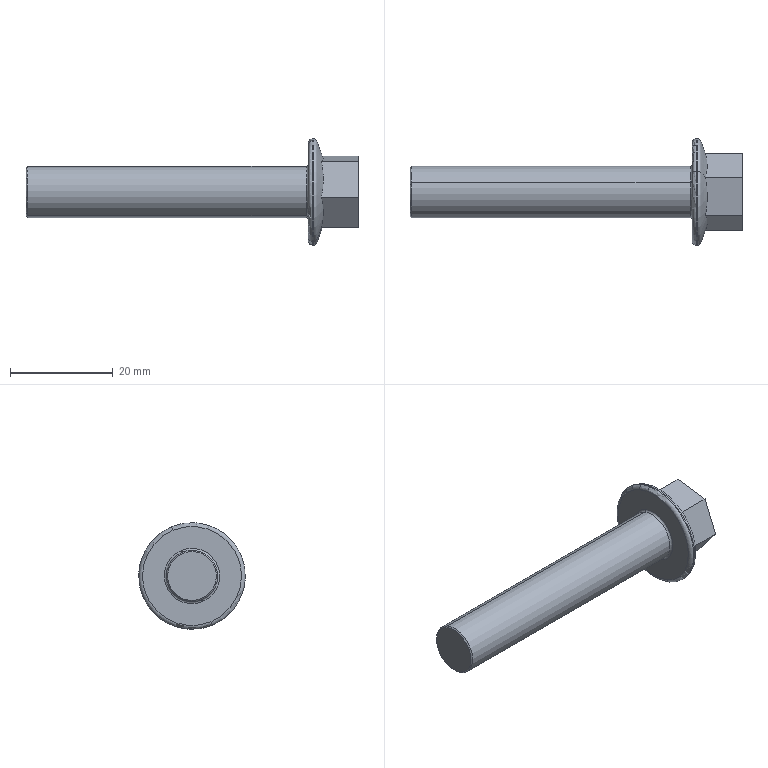Part | SolidWorks | features BaseBody 1 | 1 solid | 30 faces | box 64.7 x 20.8 x 20.8 mm | volume 6136 mm3 | cone 11 | plane 9 | torus 6 | cylinder 4 | commonest cylinder face diameters 10 x2 20.8 x2
STEP:
#1=CARTESIAN_POINT('',(181.975,42.982,433.757));
#2=VERTEX_POINT('',#1);
#3=CARTESIAN_POINT('',(181.975,35.018,414.543));
#4=VERTEX_POINT('',#3);
#5=CARTESIAN_POINT('',(181.975,39.,424.15));
#6=DIRECTION('',(-1.,0.,0.));
#7=DIRECTION('',(0.,-0.3829,-0.9238));
#8=AXIS2_PLACEMENT_3D('',#5,#6,#7);
#9=CIRCLE('',#8,10.4);
#10=EDGE_CURVE('',#2,#4,#9,.T.);
#11=ORIENTED_EDGE('',*,*,#10,.T.);
#12=CARTESIAN_POINT('',(181.75,35.018,414.543));
#13=VERTEX_POINT('',#12);
#14=CARTESIAN_POINT('',(182.5,35.018,414.543));
#15=DIRECTION('',(-1.,0.,0.));
#16=VECTOR('',#15,1000.);
#17=LINE('',#14,#16);
#18=EDGE_CURVE('',#4,#13,#17,.T.);
#19=ORIENTED_EDGE('',*,*,#18,.T.);
#20=CARTESIAN_POINT('',(181.75,42.982,433.757));
#21=VERTEX_POINT('',#20);
#22=CARTESIAN_POINT('',(181.75,39.,424.15));
#23=DIRECTION('',(1.,0.,0.));
#24=DIRECTION('',(0.,0.3829,0.9238));
#25=AXIS2_PLACEMENT_3D('',#22,#23,#24);
#26=CIRCLE('',#25,10.4);
#27=EDGE_CURVE('',#13,#21,#26,.T.);
#28=ORIENTED_EDGE('',*,*,#27,.T.);
#29=CARTESIAN_POINT('',(182.5,42.982,433.757));
#30=DIRECTION('',(-1.,0.,0.));
#31=VECTOR('',#30,1000.);
#32=LINE('',#29,#31);
#33=EDGE_CURVE('',#2,#21,#32,.T.);
#34=ORIENTED_EDGE('',*,*,#33,.F.);
#35=EDGE_LOOP('',(#11,#19,#28,#34));
#36=FACE_OUTER_BOUND('',#35,.T.);
#37=CARTESIAN_POINT('',(182.5,39.,424.15));
#38=DIRECTION('',(-1.,0.,0.));
#39=DIRECTION('',(0.,0.3829,0.9238));
#40=AXIS2_PLACEMENT_3D('',#37,#38,#39);
#41=CYLINDRICAL_SURFACE('',#40,10.4);
#42=ADVANCED_FACE('',(#36),#41,.T.);
#43=CARTESIAN_POINT('',(180.6,40.915,428.769));
#44=VERTEX_POINT('',#43);
#45=CARTESIAN_POINT('',(180.6,37.085,419.531));
#46=VERTEX_POINT('',#45);
#47=CARTESIAN_POINT('',(180.6,39.,424.15));
#48=DIRECTION('',(-1.,0.,0.));
#49=DIRECTION('',(0.,0.3829,0.9238));
#50=AXIS2_PLACEMENT_3D('',#47,#48,#49);
#51=CIRCLE('',#50,5.);
#52=EDGE_CURVE('',#44,#46,#51,.T.);
#53=ORIENTED_EDGE('',*,*,#52,.T.);
#54=CARTESIAN_POINT('',(126.25,37.085,419.531));
#55=VERTEX_POINT('',#54);
#56=CARTESIAN_POINT('',(181.,37.085,419.531));
#57=DIRECTION('',(-1.,0.,0.));
#58=VECTOR('',#57,1000.);
#59=LINE('',#56,#58);
#60=EDGE_CURVE('',#46,#55,#59,.T.);
#61=ORIENTED_EDGE('',*,*,#60,.T.);
#62=CARTESIAN_POINT('',(126.25,40.915,428.769));
#63=VERTEX_POINT('',#62);
#64=CARTESIAN_POINT('',(126.25,39.,424.15));
#65=DIRECTION('',(1.,0.,0.));
#66=DIRECTION('',(0.,0.3829,0.9238));
#67=AXIS2_PLACEMENT_3D('',#64,#65,#66);
#68=CIRCLE('',#67,5.);
#69=EDGE_CURVE('',#55,#63,#68,.T.);
#70=ORIENTED_EDGE('',*,*,#69,.T.);
#71=CARTESIAN_POINT('',(181.,40.915,428.769));
#72=DIRECTION('',(-1.,0.,0.));
#73=VECTOR('',#72,1000.);
#74=LINE('',#71,#73);
#75=EDGE_CURVE('',#44,#63,#74,.T.);
#76=ORIENTED_EDGE('',*,*,#75,.F.);
#77=EDGE_LOOP('',(#53,#61,#70,#76));
#78=FACE_OUTER_BOUND('',#77,.T.);
#79=CARTESIAN_POINT('',(181.,39.,424.15));
#80=DIRECTION('',(-1.,0.,0.));
#81=DIRECTION('',(0.,0.3829,0.9238));
#82=AXIS2_PLACEMENT_3D('',#79,#80,#81);
#83=CYLINDRICAL_SURFACE('',#82,5.);
#84=ADVANCED_FACE('',(#78),#83,.T.);
#85=CARTESIAN_POINT('',(183.553,41.874,431.083));
#86=VERTEX_POINT('',#85);
#87=CARTESIAN_POINT('',(183.553,34.432,430.106));
#88=VERTEX_POINT('',#87);
#89=CARTESIAN_POINT('',(183.553,41.874,431.083));
#90=CARTESIAN_POINT('',(183.667,41.254,431.002));
#91=CARTESIAN_POINT('',(183.76,40.634,430.921));
#92=CARTESIAN_POINT('',(183.886,39.393,430.758));
#93=CARTESIAN_POINT('',(183.953,38.153,430.595));
#94=CARTESIAN_POINT('',(183.886,36.913,430.432));
#95=CARTESIAN_POINT('',(183.76,35.673,430.269));
#96=CARTESIAN_POINT('',(183.667,35.053,430.187));
#97=CARTESIAN_POINT('',(183.553,34.432,430.106));
#98=B_SPLINE_CURVE_WITH_KNOTS('',3,(#89,#90,#91,#92,#93,#94,#95,#96,#97),.UNSPECIFIED.,.F.,.F.,(4,2,1,2,4),(0.,0.001876,0.003753,0.005629,0.007506),.UNSPECIFIED.);
#99=EDGE_CURVE('',#86,#88,#98,.T.);
#100=ORIENTED_EDGE('',*,*,#99,.F.);
#101=CARTESIAN_POINT('',(182.68,42.793,433.301));
#102=VERTEX_POINT('',#101);
#103=CARTESIAN_POINT('',(182.5,42.982,433.757));
#104=DIRECTION('',(-0.342,0.3598,0.8681));
#105=VECTOR('',#104,1000.);
#106=LINE('',#103,#105);
#107=EDGE_CURVE('',#86,#102,#106,.T.);
#108=ORIENTED_EDGE('',*,*,#107,.T.);
#109=CARTESIAN_POINT('',(182.68,35.207,414.999));
#110=VERTEX_POINT('',#109);
#111=CARTESIAN_POINT('',(182.68,39.,424.15));
#112=DIRECTION('',(1.,0.,0.));
#113=DIRECTION('',(0.,-0.3829,-0.9238));
#114=AXIS2_PLACEMENT_3D('',#111,#112,#113);
#115=CIRCLE('',#114,9.907);
#116=EDGE_CURVE('',#102,#110,#115,.T.);
#117=ORIENTED_EDGE('',*,*,#116,.T.);
#118=CARTESIAN_POINT('',(183.553,36.126,417.217));
#119=VERTEX_POINT('',#118);
#120=CARTESIAN_POINT('',(182.5,35.018,414.543));
#121=DIRECTION('',(-0.342,-0.3598,-0.8681));
#122=VECTOR('',#121,1000.);
#123=LINE('',#120,#122);
#124=EDGE_CURVE('',#119,#110,#123,.T.);
#125=ORIENTED_EDGE('',*,*,#124,.F.);
#126=CARTESIAN_POINT('',(183.553,31.558,423.172));
#127=VERTEX_POINT('',#126);
#128=CARTESIAN_POINT('',(183.553,31.558,423.172));
#129=CARTESIAN_POINT('',(183.667,31.939,422.676));
#130=CARTESIAN_POINT('',(183.76,32.32,422.18));
#131=CARTESIAN_POINT('',(183.886,33.081,421.187));
#132=CARTESIAN_POINT('',(183.953,33.842,420.194));
#133=CARTESIAN_POINT('',(183.886,34.603,419.202));
#134=CARTESIAN_POINT('',(183.76,35.365,418.209));
#135=CARTESIAN_POINT('',(183.667,35.745,417.713));
#136=CARTESIAN_POINT('',(183.553,36.126,417.217));
#137=B_SPLINE_CURVE_WITH_KNOTS('',3,(#128,#129,#130,#131,#132,#133,#134,#135,#136),.UNSPECIFIED.,.F.,.F.,(4,2,1,2,4),(0.,0.001876,0.003753,0.005629,0.007506),.UNSPECIFIED.);
#138=EDGE_CURVE('',#127,#119,#137,.T.);
#139=ORIENTED_EDGE('',*,*,#138,.F.);
#140=CARTESIAN_POINT('',(183.553,34.432,430.106));
#141=CARTESIAN_POINT('',(183.667,34.193,429.528));
#142=CARTESIAN_POINT('',(183.76,33.953,428.95));
#143=CARTESIAN_POINT('',(183.886,33.474,427.795));
#144=CARTESIAN_POINT('',(183.953,32.995,426.639));
#145=CARTESIAN_POINT('',(183.886,32.516,425.483));
#146=CARTESIAN_POINT('',(183.76,32.037,424.328));
#147=CARTESIAN_POINT('',(183.667,31.798,423.75));
#148=CARTESIAN_POINT('',(183.553,31.558,423.172));
#149=B_SPLINE_CURVE_WITH_KNOTS('',3,(#140,#141,#142,#143,#144,#145,#146,#147,#148),.UNSPECIFIED.,.F.,.F.,(4,2,1,2,4),(0.,0.001876,0.003753,0.005629,0.007506),.UNSPECIFIED.);
#150=EDGE_CURVE('',#88,#127,#149,.T.);
#151=ORIENTED_EDGE('',*,*,#150,.F.);
#152=EDGE_LOOP('',(#100,#108,#117,#125,#139,#151));
#153=FACE_OUTER_BOUND('',#152,.T.);
#154=CARTESIAN_POINT('',(182.5,39.,424.15));
#155=DIRECTION('',(-1.,0.,0.));
#156=DIRECTION('',(0.,-0.3829,-0.9238));
#157=AXIS2_PLACEMENT_3D('',#154,#155,#156);
#158=CONICAL_SURFACE('',#157,10.4,1.222);
#159=ADVANCED_FACE('',(#153),#158,.T.);
#160=CARTESIAN_POINT('',(190.7,41.863,431.082));
#161=VERTEX_POINT('',#160);
#162=CARTESIAN_POINT('',(190.7,41.872,431.078));
#163=VERTEX_POINT('',#162);
#164=CARTESIAN_POINT('',(190.7,39.,424.15));
#165=DIRECTION('',(-1.,0.,0.));
#166=DIRECTION('',(0.,0.3829,0.9238));
#167=AXIS2_PLACEMENT_3D('',#164,#165,#166);
#168=CIRCLE('',#167,7.5);
#169=EDGE_CURVE('',#161,#163,#168,.T.);
#170=ORIENTED_EDGE('',*,*,#169,.T.);
#171=CARTESIAN_POINT('',(190.697,41.874,431.083));
#172=VERTEX_POINT('',#171);
#173=CARTESIAN_POINT('',(190.7,41.872,431.078));
#174=DIRECTION('',(-0.4226,0.347,0.8372));
#175=VECTOR('',#174,1000.);
#176=LINE('',#173,#175);
#177=EDGE_CURVE('',#163,#172,#176,.T.);
#178=ORIENTED_EDGE('',*,*,#177,.T.);
#179=CARTESIAN_POINT('',(190.699,41.868,431.083));
#180=DIRECTION('',(0.2271,-0.9656,-0.1269));
#181=VECTOR('',#180,1000.);
#182=LINE('',#179,#181);
#183=EDGE_CURVE('',#172,#161,#182,.T.);
#184=ORIENTED_EDGE('',*,*,#183,.T.);
#185=EDGE_LOOP('',(#170,#178,#184));
#186=FACE_OUTER_BOUND('',#185,.T.);
#187=CARTESIAN_POINT('',(190.7,39.,424.15));
#188=DIRECTION('',(-1.,0.,0.));
#189=DIRECTION('',(0.,0.3829,0.9238));
#190=AXIS2_PLACEMENT_3D('',#187,#188,#189);
#191=CONICAL_SURFACE('',#190,7.5,1.134);
#192=ADVANCED_FACE('',(#186),#191,.T.);
#193=ORIENTED_EDGE('',*,*,#27,.F.);
#194=CARTESIAN_POINT('',(181.,35.305,415.235));
#195=VERTEX_POINT('',#194);
#196=CARTESIAN_POINT('',(181.75,35.305,415.235));
#197=DIRECTION('',(0.,0.9238,-0.3829));
#198=DIRECTION('',(0.,0.3829,0.9238));
#199=AXIS2_PLACEMENT_3D('',#196,#197,#198);
#200=CIRCLE('',#199,0.75);
#201=EDGE_CURVE('',#13,#195,#200,.T.);
#202=ORIENTED_EDGE('',*,*,#201,.T.);
#203=CARTESIAN_POINT('',(181.,42.695,433.065));
#204=VERTEX_POINT('',#203);
#205=CARTESIAN_POINT('',(181.,39.,424.15));
#206=DIRECTION('',(-1.,0.,0.));
#207=DIRECTION('',(0.,0.3829,0.9238));
#208=AXIS2_PLACEMENT_3D('',#205,#206,#207);
#209=CIRCLE('',#208,9.65);
#210=EDGE_CURVE('',#204,#195,#209,.T.);
#211=ORIENTED_EDGE('',*,*,#210,.F.);
#212=CARTESIAN_POINT('',(181.75,42.695,433.065));
#213=DIRECTION('',(0.,-0.9238,0.3829));
#214=DIRECTION('',(0.,-0.3829,-0.9238));
#215=AXIS2_PLACEMENT_3D('',#212,#213,#214);
#216=CIRCLE('',#215,0.75);
#217=EDGE_CURVE('',#21,#204,#216,.T.);
#218=ORIENTED_EDGE('',*,*,#217,.F.);
#219=EDGE_LOOP('',(#193,#202,#211,#218));
#220=FACE_OUTER_BOUND('',#219,.T.);
#221=CARTESIAN_POINT('',(181.75,39.,424.15));
#222=DIRECTION('',(-1.,0.,0.));
#223=DIRECTION('',(0.,0.3829,0.9238));
#224=AXIS2_PLACEMENT_3D('',#221,#222,#223);
#225=TOROIDAL_SURFACE('',#224,9.65,0.75);
#226=ADVANCED_FACE('',(#220),#225,.T.);
#227=ORIENTED_EDGE('',*,*,#10,.F.);
#228=CARTESIAN_POINT('',(181.975,42.695,433.065));
#229=DIRECTION('',(0.,0.9238,-0.3829));
#230=DIRECTION('',(0.,0.3829,0.9238));
#231=AXIS2_PLACEMENT_3D('',#228,#229,#230);
#232=CIRCLE('',#231,0.75);
#233=EDGE_CURVE('',#2,#102,#232,.T.);
#234=ORIENTED_EDGE('',*,*,#233,.T.);
#235=CARTESIAN_POINT('',(182.68,39.,424.15));
#236=DIRECTION('',(1.,0.,0.));
#237=DIRECTION('',(0.,-0.3829,-0.9238));
#238=AXIS2_PLACEMENT_3D('',#235,#236,#237);
#239=CIRCLE('',#238,9.907);
#240=EDGE_CURVE('',#110,#102,#239,.T.);
#241=ORIENTED_EDGE('',*,*,#240,.F.);
#242=CARTESIAN_POINT('',(181.975,35.305,415.235));
#243=DIRECTION('',(0.,-0.9238,0.3829));
#244=DIRECTION('',(0.,-0.3829,-0.9238));
#245=AXIS2_PLACEMENT_3D('',#242,#243,#244);
#246=CIRCLE('',#245,0.75);
#247=EDGE_CURVE('',#4,#110,#246,.T.);
#248=ORIENTED_EDGE('',*,*,#247,.F.);
#249=EDGE_LOOP('',(#227,#234,#241,#248));
#250=FACE_OUTER_BOUND('',#249,.T.);
#251=CARTESIAN_POINT('',(181.975,39.,424.15));
#252=DIRECTION('',(1.,0.,0.));
#253=DIRECTION('',(0.,-0.3829,-0.9238));
#254=AXIS2_PLACEMENT_3D('',#251,#252,#253);
#255=TOROIDAL_SURFACE('',#254,9.65,0.75);
#256=ADVANCED_FACE('',(#250),#255,.T.);
#257=CARTESIAN_POINT('',(180.6,39.,424.15));
#258=DIRECTION('',(-1.,0.,0.));
#259=DIRECTION('',(0.,0.3829,0.9238));
#260=AXIS2_PLACEMENT_3D('',#257,#258,#259);
#261=CIRCLE('',#260,5.);
#262=EDGE_CURVE('',#46,#44,#261,.T.);
#263=ORIENTED_EDGE('',*,*,#262,.F.);
#264=CARTESIAN_POINT('',(181.,36.932,419.162));
#265=VERTEX_POINT('',#264);
#266=CARTESIAN_POINT('',(180.6,36.932,419.162));
#267=DIRECTION('',(0.,0.9238,-0.3829));
#268=DIRECTION('',(0.,0.3829,0.9238));
#269=AXIS2_PLACEMENT_3D('',#266,#267,#268);
#270=CIRCLE('',#269,0.4);
#271=EDGE_CURVE('',#46,#265,#270,.T.);
#272=ORIENTED_EDGE('',*,*,#271,.T.);
#273=CARTESIAN_POINT('',(181.,41.068,429.138));
#274=VERTEX_POINT('',#273);
#275=CARTESIAN_POINT('',(181.,39.,424.15));
#276=DIRECTION('',(1.,0.,0.));
#277=DIRECTION('',(0.,0.3829,0.9238));
#278=AXIS2_PLACEMENT_3D('',#275,#276,#277);
#279=CIRCLE('',#278,5.4);
#280=EDGE_CURVE('',#274,#265,#279,.T.);
#281=ORIENTED_EDGE('',*,*,#280,.F.);
#282=CARTESIAN_POINT('',(180.6,41.068,429.138));
#283=DIRECTION('',(0.,-0.9238,0.3829));
#284=DIRECTION('',(0.,-0.3829,-0.9238));
#285=AXIS2_PLACEMENT_3D('',#282,#283,#284);
#286=CIRCLE('',#285,0.4);
#287=EDGE_CURVE('',#44,#274,#286,.T.);
#288=ORIENTED_EDGE('',*,*,#287,.F.);
#289=EDGE_LOOP('',(#263,#272,#281,#288));
#290=FACE_OUTER_BOUND('',#289,.T.);
#291=CARTESIAN_POINT('',(180.6,39.,424.15));
#292=DIRECTION('',(-1.,0.,0.));
#293=DIRECTION('',(0.,0.3829,0.9238));
#294=AXIS2_PLACEMENT_3D('',#291,#292,#293);
#295=TOROIDAL_SURFACE('',#294,5.4,0.4);
#296=ADVANCED_FACE('',(#290),#295,.F.);
#297=CARTESIAN_POINT('',(126.,40.819,428.538));
#298=VERTEX_POINT('',#297);
#299=CARTESIAN_POINT('',(126.,37.181,419.762));
#300=VERTEX_POINT('',#299);
#301=CARTESIAN_POINT('',(126.,39.,424.15));
#302=DIRECTION('',(-1.,0.,0.));
#303=DIRECTION('',(0.,0.3829,0.9238));
#304=AXIS2_PLACEMENT_3D('',#301,#302,#303);
#305=CIRCLE('',#304,4.75);
#306=EDGE_CURVE('',#298,#300,#305,.T.);
#307=ORIENTED_EDGE('',*,*,#306,.F.);
#308=CARTESIAN_POINT('',(126.,40.819,428.538));
#309=DIRECTION('',(0.7071,0.2708,0.6532));
#310=VECTOR('',#309,1000.);
#311=LINE('',#308,#310);
#312=EDGE_CURVE('',#298,#63,#311,.T.);
#313=ORIENTED_EDGE('',*,*,#312,.T.);
#314=ORIENTED_EDGE('',*,*,#69,.F.);
#315=CARTESIAN_POINT('',(126.,37.181,419.762));
#316=DIRECTION('',(0.7071,-0.2708,-0.6532));
#317=VECTOR('',#316,1000.);
#318=LINE('',#315,#317);
#319=EDGE_CURVE('',#300,#55,#318,.T.);
#320=ORIENTED_EDGE('',*,*,#319,.F.);
#321=EDGE_LOOP('',(#307,#313,#314,#320));
#322=FACE_OUTER_BOUND('',#321,.T.);
#323=CARTESIAN_POINT('',(126.,39.,424.15));
#324=DIRECTION('',(1.,0.,0.));
#325=DIRECTION('',(0.,-0.3829,-0.9238));
#326=AXIS2_PLACEMENT_3D('',#323,#324,#325);
#327=CONICAL_SURFACE('',#326,4.75,0.7854);
#328=ADVANCED_FACE('',(#322),#327,.T.);
#329=ORIENTED_EDGE('',*,*,#312,.F.);
#330=CARTESIAN_POINT('',(126.,39.,424.15));
#331=DIRECTION('',(-1.,0.,0.));
#332=DIRECTION('',(0.,0.3829,0.9238));
#333=AXIS2_PLACEMENT_3D('',#330,#331,#332);
#334=CIRCLE('',#333,4.75);
#335=EDGE_CURVE('',#300,#298,#334,.T.);
#336=ORIENTED_EDGE('',*,*,#335,.F.);
#337=ORIENTED_EDGE('',*,*,#319,.T.);
#338=CARTESIAN_POINT('',(126.25,39.,424.15));
#339=DIRECTION('',(1.,0.,0.));
#340=DIRECTION('',(0.,0.3829,0.9238));
#341=AXIS2_PLACEMENT_3D('',#338,#339,#340);
#342=CIRCLE('',#341,5.);
#343=EDGE_CURVE('',#63,#55,#342,.T.);
#344=ORIENTED_EDGE('',*,*,#343,.F.);
#345=EDGE_LOOP('',(#329,#336,#337,#344));
#346=FACE_OUTER_BOUND('',#345,.T.);
#347=CARTESIAN_POINT('',(126.,39.,424.15));
#348=DIRECTION('',(1.,0.,0.));
#349=DIRECTION('',(0.,-0.3829,-0.9238));
#350=AXIS2_PLACEMENT_3D('',#347,#348,#349);
#351=CONICAL_SURFACE('',#350,4.75,0.7854);
#352=ADVANCED_FACE('',(#346),#351,.T.);
#353=ORIENTED_EDGE('',*,*,#271,.F.);
#354=ORIENTED_EDGE('',*,*,#52,.F.);
#355=ORIENTED_EDGE('',*,*,#287,.T.);
#356=CARTESIAN_POINT('',(181.,39.,424.15));
#357=DIRECTION('',(1.,0.,0.));
#358=DIRECTION('',(0.,0.3829,0.9238));
#359=AXIS2_PLACEMENT_3D('',#356,#357,#358);
#360=CIRCLE('',#359,5.4);
#361=EDGE_CURVE('',#265,#274,#360,.T.);
#362=ORIENTED_EDGE('',*,*,#361,.F.);
#363=EDGE_LOOP('',(#353,#354,#355,#362));
#364=FACE_OUTER_BOUND('',#363,.T.);
#365=CARTESIAN_POINT('',(180.6,39.,424.15));
#366=DIRECTION('',(-1.,0.,0.));
#367=DIRECTION('',(0.,0.3829,0.9238));
#368=AXIS2_PLACEMENT_3D('',#365,#366,#367);
#369=TOROIDAL_SURFACE('',#368,5.4,0.4);
#370=ADVANCED_FACE('',(#364),#369,.F.);
#371=ORIENTED_EDGE('',*,*,#233,.F.);
#372=CARTESIAN_POINT('',(181.975,39.,424.15));
#373=DIRECTION('',(-1.,0.,0.));
#374=DIRECTION('',(0.,-0.3829,-0.9238));
#375=AXIS2_PLACEMENT_3D('',#372,#373,#374);
#376=CIRCLE('',#375,10.4);
#377=EDGE_CURVE('',#4,#2,#376,.T.);
#378=ORIENTED_EDGE('',*,*,#377,.F.);
#379=ORIENTED_EDGE('',*,*,#247,.T.);
#380=ORIENTED_EDGE('',*,*,#116,.F.);
#381=EDGE_LOOP('',(#371,#378,#379,#380));
#382=FACE_OUTER_BOUND('',#381,.T.);
#383=CARTESIAN_POINT('',(181.975,39.,424.15));
#384=DIRECTION('',(1.,0.,0.));
#385=DIRECTION('',(0.,-0.3829,-0.9238));
#386=AXIS2_PLACEMENT_3D('',#383,#384,#385);
#387=TOROIDAL_SURFACE('',#386,9.65,0.75);
#388=ADVANCED_FACE('',(#382),#387,.T.);
#389=ORIENTED_EDGE('',*,*,#201,.F.);
#390=CARTESIAN_POINT('',(181.75,39.,424.15));
#391=DIRECTION('',(1.,0.,0.));
#392=DIRECTION('',(0.,0.3829,0.9238));
#393=AXIS2_PLACEMENT_3D('',#390,#391,#392);
#394=CIRCLE('',#393,10.4);
#395=EDGE_CURVE('',#21,#13,#394,.T.);
#396=ORIENTED_EDGE('',*,*,#395,.F.);
#397=ORIENTED_EDGE('',*,*,#217,.T.);
#398=CARTESIAN_POINT('',(181.,39.,424.15));
#399=DIRECTION('',(-1.,0.,0.));
#400=DIRECTION('',(0.,0.3829,0.9238));
#401=AXIS2_PLACEMENT_3D('',#398,#399,#400);
#402=CIRCLE('',#401,9.65);
#403=EDGE_CURVE('',#195,#204,#402,.T.);
#404=ORIENTED_EDGE('',*,*,#403,.F.);
#405=EDGE_LOOP('',(#389,#396,#397,#404));
#406=FACE_OUTER_BOUND('',#405,.T.);
#407=CARTESIAN_POINT('',(181.75,39.,424.15));
#408=DIRECTION('',(-1.,0.,0.));
#409=DIRECTION('',(0.,0.3829,0.9238));
#410=AXIS2_PLACEMENT_3D('',#407,#408,#409);
#411=TOROIDAL_SURFACE('',#410,9.65,0.75);
#412=ADVANCED_FACE('',(#406),#411,.T.);
#413=CARTESIAN_POINT('',(190.697,36.126,417.217));
#414=VERTEX_POINT('',#413);
#415=CARTESIAN_POINT('',(190.7,36.137,417.218));
#416=VERTEX_POINT('',#415);
#417=CARTESIAN_POINT('',(190.699,36.132,417.217));
#418=DIRECTION('',(0.2271,0.9656,0.1269));
#419=VECTOR('',#418,1000.);
#420=LINE('',#417,#419);
#421=EDGE_CURVE('',#414,#416,#420,.T.);
#422=ORIENTED_EDGE('',*,*,#421,.T.);
#423=CARTESIAN_POINT('',(190.7,36.119,417.225));
#424=VERTEX_POINT('',#423);
#425=CARTESIAN_POINT('',(190.7,39.,424.15));
#426=DIRECTION('',(-1.,0.,0.));
#427=DIRECTION('',(0.,0.3829,0.9238));
#428=AXIS2_PLACEMENT_3D('',#425,#426,#427);
#429=CIRCLE('',#428,7.5);
#430=EDGE_CURVE('',#416,#424,#429,.T.);
#431=ORIENTED_EDGE('',*,*,#430,.T.);
#432=CARTESIAN_POINT('',(190.699,36.123,417.221));
#433=DIRECTION('',(-0.2266,0.5927,-0.7729));
#434=VECTOR('',#433,1000.);
#435=LINE('',#432,#434);
#436=EDGE_CURVE('',#424,#414,#435,.T.);
#437=ORIENTED_EDGE('',*,*,#436,.T.);
#438=EDGE_LOOP('',(#422,#431,#437));
#439=FACE_OUTER_BOUND('',#438,.T.);
#440=CARTESIAN_POINT('',(190.7,39.,424.15));
#441=DIRECTION('',(-1.,0.,0.));
#442=DIRECTION('',(0.,0.3829,0.9238));
#443=AXIS2_PLACEMENT_3D('',#440,#441,#442);
#444=CONICAL_SURFACE('',#443,7.5,1.134);
#445=ADVANCED_FACE('',(#439),#444,.T.);
#446=CARTESIAN_POINT('',(190.697,43.568,418.194));
#447=VERTEX_POINT('',#446);
#448=CARTESIAN_POINT('',(190.7,43.572,418.205));
#449=VERTEX_POINT('',#448);
#450=CARTESIAN_POINT('',(190.699,43.57,418.199));
#451=DIRECTION('',(0.2271,0.3729,0.8997));
#452=VECTOR('',#451,1000.);
#453=LINE('',#450,#452);
#454=EDGE_CURVE('',#447,#449,#453,.T.);
#455=ORIENTED_EDGE('',*,*,#454,.T.);
#456=CARTESIAN_POINT('',(190.7,43.557,418.193));
#457=VERTEX_POINT('',#456);
#458=CARTESIAN_POINT('',(190.7,39.,424.15));
#459=DIRECTION('',(-1.,0.,0.));
#460=DIRECTION('',(0.,0.3829,0.9238));
#461=AXIS2_PLACEMENT_3D('',#458,#459,#460);
#462=CIRCLE('',#461,7.5);
#463=EDGE_CURVE('',#449,#457,#462,.T.);
#464=ORIENTED_EDGE('',*,*,#463,.T.);
#465=CARTESIAN_POINT('',(190.699,43.562,418.194));
#466=DIRECTION('',(-0.2266,0.9657,0.1269));
#467=VECTOR('',#466,1000.);
#468=LINE('',#465,#467);
#469=EDGE_CURVE('',#457,#447,#468,.T.);
#470=ORIENTED_EDGE('',*,*,#469,.T.);
#471=EDGE_LOOP('',(#455,#464,#470));
#472=FACE_OUTER_BOUND('',#471,.T.);
#473=CARTESIAN_POINT('',(190.7,39.,424.15));
#474=DIRECTION('',(-1.,0.,0.));
#475=DIRECTION('',(0.,0.3829,0.9238));
#476=AXIS2_PLACEMENT_3D('',#473,#474,#475);
#477=CONICAL_SURFACE('',#476,7.5,1.134);
#478=ADVANCED_FACE('',(#472),#477,.T.);
#479=CARTESIAN_POINT('',(190.697,46.442,425.128));
#480=VERTEX_POINT('',#479);
#481=CARTESIAN_POINT('',(190.7,46.435,425.137));
#482=VERTEX_POINT('',#481);
#483=CARTESIAN_POINT('',(190.699,46.438,425.132));
#484=DIRECTION('',(0.2271,-0.5927,0.7728));
#485=VECTOR('',#484,1000.);
#486=LINE('',#483,#485);
#487=EDGE_CURVE('',#480,#482,#486,.T.);
#488=ORIENTED_EDGE('',*,*,#487,.T.);
#489=CARTESIAN_POINT('',(190.7,46.437,425.118));
#490=VERTEX_POINT('',#489);
#491=CARTESIAN_POINT('',(190.7,39.,424.15));
#492=DIRECTION('',(-1.,0.,0.));
#493=DIRECTION('',(0.,0.3829,0.9238));
#494=AXIS2_PLACEMENT_3D('',#491,#492,#493);
#495=CIRCLE('',#494,7.5);
#496=EDGE_CURVE('',#482,#490,#495,.T.);
#497=ORIENTED_EDGE('',*,*,#496,.T.);
#498=CARTESIAN_POINT('',(190.699,46.439,425.123));
#499=DIRECTION('',(-0.2266,0.373,0.8998));
#500=VECTOR('',#499,1000.);
#501=LINE('',#498,#500);
#502=EDGE_CURVE('',#490,#480,#501,.T.);
#503=ORIENTED_EDGE('',*,*,#502,.T.);
#504=EDGE_LOOP('',(#488,#497,#503));
#505=FACE_OUTER_BOUND('',#504,.T.);
#506=CARTESIAN_POINT('',(190.7,39.,424.15));
#507=DIRECTION('',(-1.,0.,0.));
#508=DIRECTION('',(0.,0.3829,0.9238));
#509=AXIS2_PLACEMENT_3D('',#506,#507,#508);
#510=CONICAL_SURFACE('',#509,7.5,1.134);
#511=ADVANCED_FACE('',(#505),#510,.T.);
#512=ORIENTED_EDGE('',*,*,#177,.F.);
#513=CARTESIAN_POINT('',(190.7,41.881,431.075));
#514=VERTEX_POINT('',#513);
#515=CARTESIAN_POINT('',(190.7,39.,424.15));
#516=DIRECTION('',(-1.,0.,0.));
#517=DIRECTION('',(0.,0.3829,0.9238));
#518=AXIS2_PLACEMENT_3D('',#515,#516,#517);
#519=CIRCLE('',#518,7.5);
#520=EDGE_CURVE('',#163,#514,#519,.T.);
#521=ORIENTED_EDGE('',*,*,#520,.T.);
#522=CARTESIAN_POINT('',(190.699,41.877,431.079));
#523=DIRECTION('',(-0.2266,-0.5927,0.7729));
#524=VECTOR('',#523,1000.);
#525=LINE('',#522,#524);
#526=EDGE_CURVE('',#514,#172,#525,.T.);
#527=ORIENTED_EDGE('',*,*,#526,.T.);
#528=EDGE_LOOP('',(#512,#521,#527));
#529=FACE_OUTER_BOUND('',#528,.T.);
#530=CARTESIAN_POINT('',(190.7,39.,424.15));
#531=DIRECTION('',(-1.,0.,0.));
#532=DIRECTION('',(0.,0.3829,0.9238));
#533=AXIS2_PLACEMENT_3D('',#530,#531,#532);
#534=CONICAL_SURFACE('',#533,7.5,1.134);
#535=ADVANCED_FACE('',(#529),#534,.T.);
#536=CARTESIAN_POINT('',(190.697,34.432,430.106));
#537=VERTEX_POINT('',#536);
#538=CARTESIAN_POINT('',(190.7,34.428,430.095));
#539=VERTEX_POINT('',#538);
#540=CARTESIAN_POINT('',(190.699,34.43,430.101));
#541=DIRECTION('',(0.2271,-0.3729,-0.8997));
#542=VECTOR('',#541,1000.);
#543=LINE('',#540,#542);
#544=EDGE_CURVE('',#537,#539,#543,.T.);
#545=ORIENTED_EDGE('',*,*,#544,.T.);
#546=CARTESIAN_POINT('',(190.7,34.443,430.107));
#547=VERTEX_POINT('',#546);
#548=CARTESIAN_POINT('',(190.7,39.,424.15));
#549=DIRECTION('',(-1.,0.,0.));
#550=DIRECTION('',(0.,0.3829,0.9238));
#551=AXIS2_PLACEMENT_3D('',#548,#549,#550);
#552=CIRCLE('',#551,7.5);
#553=EDGE_CURVE('',#539,#547,#552,.T.);
#554=ORIENTED_EDGE('',*,*,#553,.T.);
#555=CARTESIAN_POINT('',(190.699,34.438,430.106));
#556=DIRECTION('',(-0.2266,-0.9657,-0.1269));
#557=VECTOR('',#556,1000.);
#558=LINE('',#555,#557);
#559=EDGE_CURVE('',#547,#537,#558,.T.);
#560=ORIENTED_EDGE('',*,*,#559,.T.);
#561=EDGE_LOOP('',(#545,#554,#560));
#562=FACE_OUTER_BOUND('',#561,.T.);
#563=CARTESIAN_POINT('',(190.7,39.,424.15));
#564=DIRECTION('',(-1.,0.,0.));
#565=DIRECTION('',(0.,0.3829,0.9238));
#566=AXIS2_PLACEMENT_3D('',#563,#564,#565);
#567=CONICAL_SURFACE('',#566,7.5,1.134);
#568=ADVANCED_FACE('',(#562),#567,.T.);
#569=CARTESIAN_POINT('',(190.697,31.558,423.172));
#570=VERTEX_POINT('',#569);
#571=CARTESIAN_POINT('',(190.7,31.565,423.163));
#572=VERTEX_POINT('',#571);
#573=CARTESIAN_POINT('',(190.699,31.562,423.168));
#574=DIRECTION('',(0.2271,0.5927,-0.7728));
#575=VECTOR('',#574,1000.);
#576=LINE('',#573,#575);
#577=EDGE_CURVE('',#570,#572,#576,.T.);
#578=ORIENTED_EDGE('',*,*,#577,.T.);
#579=CARTESIAN_POINT('',(190.7,31.563,423.182));
#580=VERTEX_POINT('',#579);
#581=CARTESIAN_POINT('',(190.7,39.,424.15));
#582=DIRECTION('',(-1.,0.,0.));
#583=DIRECTION('',(0.,0.3829,0.9238));
#584=AXIS2_PLACEMENT_3D('',#581,#582,#583);
#585=CIRCLE('',#584,7.5);
#586=EDGE_CURVE('',#572,#580,#585,.T.);
#587=ORIENTED_EDGE('',*,*,#586,.T.);
#588=CARTESIAN_POINT('',(190.699,31.561,423.177));
#589=DIRECTION('',(-0.2266,-0.373,-0.8998));
#590=VECTOR('',#589,1000.);
#591=LINE('',#588,#590);
#592=EDGE_CURVE('',#580,#570,#591,.T.);
#593=ORIENTED_EDGE('',*,*,#592,.T.);
#594=EDGE_LOOP('',(#578,#587,#593));
#595=FACE_OUTER_BOUND('',#594,.T.);
#596=CARTESIAN_POINT('',(190.7,39.,424.15));
#597=DIRECTION('',(-1.,0.,0.));
#598=DIRECTION('',(0.,0.3829,0.9238));
#599=AXIS2_PLACEMENT_3D('',#596,#597,#598);
#600=CONICAL_SURFACE('',#599,7.5,1.134);
#601=ADVANCED_FACE('',(#595),#600,.T.);
#602=ORIENTED_EDGE('',*,*,#107,.F.);
#603=CARTESIAN_POINT('',(183.553,46.442,425.128));
#604=VERTEX_POINT('',#603);
#605=CARTESIAN_POINT('',(183.553,46.442,425.128));
#606=CARTESIAN_POINT('',(183.667,46.061,425.624));
#607=CARTESIAN_POINT('',(183.76,45.68,426.12));
#608=CARTESIAN_POINT('',(183.886,44.919,427.113));
#609=CARTESIAN_POINT('',(183.953,44.158,428.106));
#610=CARTESIAN_POINT('',(183.886,43.397,429.098));
#611=CARTESIAN_POINT('',(183.76,42.635,430.091));
#612=CARTESIAN_POINT('',(183.667,42.255,430.587));
#613=CARTESIAN_POINT('',(183.553,41.874,431.083));
#614=B_SPLINE_CURVE_WITH_KNOTS('',3,(#605,#606,#607,#608,#609,#610,#611,#612,#613),.UNSPECIFIED.,.F.,.F.,(4,2,1,2,4),(0.,0.001876,0.003753,0.005629,0.007506),.UNSPECIFIED.);
#615=EDGE_CURVE('',#604,#86,#614,.T.);
#616=ORIENTED_EDGE('',*,*,#615,.F.);
#617=CARTESIAN_POINT('',(183.553,43.568,418.194));
#618=VERTEX_POINT('',#617);
#619=CARTESIAN_POINT('',(183.553,43.568,418.194));
#620=CARTESIAN_POINT('',(183.667,43.807,418.772));
#621=CARTESIAN_POINT('',(183.76,44.047,419.35));
#622=CARTESIAN_POINT('',(183.886,44.526,420.505));
#623=CARTESIAN_POINT('',(183.953,45.005,421.661));
#624=CARTESIAN_POINT('',(183.886,45.484,422.817));
#625=CARTESIAN_POINT('',(183.76,45.963,423.972));
#626=CARTESIAN_POINT('',(183.667,46.202,424.55));
#627=CARTESIAN_POINT('',(183.553,46.442,425.128));
#628=B_SPLINE_CURVE_WITH_KNOTS('',3,(#619,#620,#621,#622,#623,#624,#625,#626,#627),.UNSPECIFIED.,.F.,.F.,(4,2,1,2,4),(0.,0.001876,0.003753,0.005629,0.007506),.UNSPECIFIED.);
#629=EDGE_CURVE('',#618,#604,#628,.T.);
#630=ORIENTED_EDGE('',*,*,#629,.F.);
#631=CARTESIAN_POINT('',(183.553,36.126,417.217));
#632=CARTESIAN_POINT('',(183.667,36.746,417.298));
#633=CARTESIAN_POINT('',(183.76,37.366,417.379));
#634=CARTESIAN_POINT('',(183.886,38.607,417.542));
#635=CARTESIAN_POINT('',(183.953,39.847,417.705));
#636=CARTESIAN_POINT('',(183.886,41.087,417.868));
#637=CARTESIAN_POINT('',(183.76,42.327,418.031));
#638=CARTESIAN_POINT('',(183.667,42.947,418.113));
#639=CARTESIAN_POINT('',(183.553,43.568,418.194));
#640=B_SPLINE_CURVE_WITH_KNOTS('',3,(#631,#632,#633,#634,#635,#636,#637,#638,#639),.UNSPECIFIED.,.F.,.F.,(4,2,1,2,4),(0.,0.001876,0.003753,0.005629,0.007506),.UNSPECIFIED.);
#641=EDGE_CURVE('',#119,#618,#640,.T.);
#642=ORIENTED_EDGE('',*,*,#641,.F.);
#643=ORIENTED_EDGE('',*,*,#124,.T.);
#644=ORIENTED_EDGE('',*,*,#240,.T.);
#645=EDGE_LOOP('',(#602,#616,#630,#642,#643,#644));
#646=FACE_OUTER_BOUND('',#645,.T.);
#647=CARTESIAN_POINT('',(182.5,39.,424.15));
#648=DIRECTION('',(-1.,0.,0.));
#649=DIRECTION('',(0.,-0.3829,-0.9238));
#650=AXIS2_PLACEMENT_3D('',#647,#648,#649);
#651=CONICAL_SURFACE('',#650,10.4,1.222);
#652=ADVANCED_FACE('',(#646),#651,.T.);
#653=ORIENTED_EDGE('',*,*,#60,.F.);
#654=ORIENTED_EDGE('',*,*,#262,.T.);
#655=ORIENTED_EDGE('',*,*,#75,.T.);
#656=ORIENTED_EDGE('',*,*,#343,.T.);
#657=EDGE_LOOP('',(#653,#654,#655,#656));
#658=FACE_OUTER_BOUND('',#657,.T.);
#659=CARTESIAN_POINT('',(181.,39.,424.15));
#660=DIRECTION('',(-1.,0.,0.));
#661=DIRECTION('',(0.,0.3829,0.9238));
#662=AXIS2_PLACEMENT_3D('',#659,#660,#661);
#663=CYLINDRICAL_SURFACE('',#662,5.);
#664=ADVANCED_FACE('',(#658),#663,.T.);
#665=ORIENTED_EDGE('',*,*,#335,.T.);
#666=ORIENTED_EDGE('',*,*,#306,.T.);
#667=EDGE_LOOP('',(#665,#666));
#668=FACE_OUTER_BOUND('',#667,.T.);
#669=CARTESIAN_POINT('',(126.,39.,424.15));
#670=DIRECTION('',(-1.,0.,0.));
#671=DIRECTION('',(0.,0.,1.));
#672=AXIS2_PLACEMENT_3D('',#669,#670,#671);
#673=PLANE('',#672);
#674=ADVANCED_FACE('',(#668),#673,.T.);
#675=ORIENTED_EDGE('',*,*,#18,.F.);
#676=ORIENTED_EDGE('',*,*,#377,.T.);
#677=ORIENTED_EDGE('',*,*,#33,.T.);
#678=ORIENTED_EDGE('',*,*,#395,.T.);
#679=EDGE_LOOP('',(#675,#676,#677,#678));
#680=FACE_OUTER_BOUND('',#679,.T.);
#681=CARTESIAN_POINT('',(182.5,39.,424.15));
#682=DIRECTION('',(-1.,0.,0.));
#683=DIRECTION('',(0.,0.3829,0.9238));
#684=AXIS2_PLACEMENT_3D('',#681,#682,#683);
#685=CYLINDRICAL_SURFACE('',#684,10.4);
#686=ADVANCED_FACE('',(#680),#685,.T.);
#687=ORIENTED_EDGE('',*,*,#210,.T.);
#688=ORIENTED_EDGE('',*,*,#403,.T.);
#689=EDGE_LOOP('',(#687,#688));
#690=FACE_OUTER_BOUND('',#689,.T.);
#691=ORIENTED_EDGE('',*,*,#280,.T.);
#692=ORIENTED_EDGE('',*,*,#361,.T.);
#693=EDGE_LOOP('',(#691,#692));
#694=FACE_BOUND('',#693,.T.);
#695=CARTESIAN_POINT('',(181.,39.,424.15));
#696=DIRECTION('',(-1.,0.,0.));
#697=DIRECTION('',(0.,0.,1.));
#698=AXIS2_PLACEMENT_3D('',#695,#696,#697);
#699=PLANE('',#698);
#700=ADVANCED_FACE('',(#690,#694),#699,.T.);
#701=ORIENTED_EDGE('',*,*,#544,.F.);
#702=CARTESIAN_POINT('',(182.5,34.432,430.106));
#703=DIRECTION('',(1.,0.,0.));
#704=VECTOR('',#703,1000.);
#705=LINE('',#702,#704);
#706=EDGE_CURVE('',#88,#537,#705,.T.);
#707=ORIENTED_EDGE('',*,*,#706,.F.);
#708=ORIENTED_EDGE('',*,*,#150,.T.);
#709=CARTESIAN_POINT('',(182.5,31.558,423.172));
#710=DIRECTION('',(1.,0.,0.));
#711=VECTOR('',#710,1000.);
#712=LINE('',#709,#711);
#713=EDGE_CURVE('',#127,#570,#712,.T.);
#714=ORIENTED_EDGE('',*,*,#713,.T.);
#715=ORIENTED_EDGE('',*,*,#592,.F.);
#716=CARTESIAN_POINT('',(190.7,31.558,423.172));
#717=DIRECTION('',(0.,0.3829,0.9238));
#718=VECTOR('',#717,1000.);
#719=LINE('',#716,#718);
#720=EDGE_CURVE('',#580,#539,#719,.T.);
#721=ORIENTED_EDGE('',*,*,#720,.T.);
#722=EDGE_LOOP('',(#701,#707,#708,#714,#715,#721));
#723=FACE_OUTER_BOUND('',#722,.T.);
#724=CARTESIAN_POINT('',(182.5,31.558,423.172));
#725=DIRECTION('',(0.,0.9238,-0.3829));
#726=DIRECTION('',(-1.,0.,0.));
#727=AXIS2_PLACEMENT_3D('',#724,#725,#726);
#728=PLANE('',#727);
#729=ADVANCED_FACE('',(#723),#728,.F.);
#730=ORIENTED_EDGE('',*,*,#183,.F.);
#731=CARTESIAN_POINT('',(182.5,41.874,431.083));
#732=DIRECTION('',(1.,0.,0.));
#733=VECTOR('',#732,1000.);
#734=LINE('',#731,#733);
#735=EDGE_CURVE('',#86,#172,#734,.T.);
#736=ORIENTED_EDGE('',*,*,#735,.F.);
#737=ORIENTED_EDGE('',*,*,#99,.T.);
#738=ORIENTED_EDGE('',*,*,#706,.T.);
#739=ORIENTED_EDGE('',*,*,#559,.F.);
#740=CARTESIAN_POINT('',(190.7,34.432,430.106));
#741=DIRECTION('',(0.,0.9915,0.1303));
#742=VECTOR('',#741,1000.);
#743=LINE('',#740,#742);
#744=EDGE_CURVE('',#547,#161,#743,.T.);
#745=ORIENTED_EDGE('',*,*,#744,.T.);
#746=EDGE_LOOP('',(#730,#736,#737,#738,#739,#745));
#747=FACE_OUTER_BOUND('',#746,.T.);
#748=CARTESIAN_POINT('',(182.5,34.432,430.106));
#749=DIRECTION('',(0.,0.1303,-0.9915));
#750=DIRECTION('',(-1.,0.,0.));
#751=AXIS2_PLACEMENT_3D('',#748,#749,#750);
#752=PLANE('',#751);
#753=ADVANCED_FACE('',(#747),#752,.F.);
#754=ORIENTED_EDGE('',*,*,#487,.F.);
#755=CARTESIAN_POINT('',(182.5,46.442,425.128));
#756=DIRECTION('',(1.,0.,0.));
#757=VECTOR('',#756,1000.);
#758=LINE('',#755,#757);
#759=EDGE_CURVE('',#604,#480,#758,.T.);
#760=ORIENTED_EDGE('',*,*,#759,.F.);
#761=ORIENTED_EDGE('',*,*,#615,.T.);
#762=ORIENTED_EDGE('',*,*,#735,.T.);
#763=ORIENTED_EDGE('',*,*,#526,.F.);
#764=CARTESIAN_POINT('',(190.7,41.874,431.083));
#765=DIRECTION('',(0.,0.6086,-0.7935));
#766=VECTOR('',#765,1000.);
#767=LINE('',#764,#766);
#768=EDGE_CURVE('',#514,#482,#767,.T.);
#769=ORIENTED_EDGE('',*,*,#768,.T.);
#770=EDGE_LOOP('',(#754,#760,#761,#762,#763,#769));
#771=FACE_OUTER_BOUND('',#770,.T.);
#772=CARTESIAN_POINT('',(182.5,41.874,431.083));
#773=DIRECTION('',(0.,-0.7935,-0.6086));
#774=DIRECTION('',(0.,0.6086,-0.7935));
#775=AXIS2_PLACEMENT_3D('',#772,#773,#774);
#776=PLANE('',#775);
#777=ADVANCED_FACE('',(#771),#776,.F.);
#778=ORIENTED_EDGE('',*,*,#454,.F.);
#779=CARTESIAN_POINT('',(182.5,43.568,418.194));
#780=DIRECTION('',(1.,0.,0.));
#781=VECTOR('',#780,1000.);
#782=LINE('',#779,#781);
#783=EDGE_CURVE('',#618,#447,#782,.T.);
#784=ORIENTED_EDGE('',*,*,#783,.F.);
#785=ORIENTED_EDGE('',*,*,#629,.T.);
#786=ORIENTED_EDGE('',*,*,#759,.T.);
#787=ORIENTED_EDGE('',*,*,#502,.F.);
#788=CARTESIAN_POINT('',(190.7,46.442,425.128));
#789=DIRECTION('',(0.,-0.3829,-0.9238));
#790=VECTOR('',#789,1000.);
#791=LINE('',#788,#790);
#792=EDGE_CURVE('',#490,#449,#791,.T.);
#793=ORIENTED_EDGE('',*,*,#792,.T.);
#794=EDGE_LOOP('',(#778,#784,#785,#786,#787,#793));
#795=FACE_OUTER_BOUND('',#794,.T.);
#796=CARTESIAN_POINT('',(182.5,46.442,425.128));
#797=DIRECTION('',(0.,-0.9238,0.3829));
#798=DIRECTION('',(-1.,0.,0.));
#799=AXIS2_PLACEMENT_3D('',#796,#797,#798);
#800=PLANE('',#799);
#801=ADVANCED_FACE('',(#795),#800,.F.);
#802=ORIENTED_EDGE('',*,*,#421,.F.);
#803=CARTESIAN_POINT('',(182.5,36.126,417.217));
#804=DIRECTION('',(1.,0.,0.));
#805=VECTOR('',#804,1000.);
#806=LINE('',#803,#805);
#807=EDGE_CURVE('',#119,#414,#806,.T.);
#808=ORIENTED_EDGE('',*,*,#807,.F.);
#809=ORIENTED_EDGE('',*,*,#641,.T.);
#810=ORIENTED_EDGE('',*,*,#783,.T.);
#811=ORIENTED_EDGE('',*,*,#469,.F.);
#812=CARTESIAN_POINT('',(190.7,43.568,418.194));
#813=DIRECTION('',(0.,-0.9915,-0.1303));
#814=VECTOR('',#813,1000.);
#815=LINE('',#812,#814);
#816=EDGE_CURVE('',#457,#416,#815,.T.);
#817=ORIENTED_EDGE('',*,*,#816,.T.);
#818=EDGE_LOOP('',(#802,#808,#809,#810,#811,#817));
#819=FACE_OUTER_BOUND('',#818,.T.);
#820=CARTESIAN_POINT('',(182.5,43.568,418.194));
#821=DIRECTION('',(0.,-0.1303,0.9915));
#822=DIRECTION('',(-1.,0.,0.));
#823=AXIS2_PLACEMENT_3D('',#820,#821,#822);
#824=PLANE('',#823);
#825=ADVANCED_FACE('',(#819),#824,.F.);
#826=ORIENTED_EDGE('',*,*,#577,.F.);
#827=ORIENTED_EDGE('',*,*,#713,.F.);
#828=ORIENTED_EDGE('',*,*,#138,.T.);
#829=ORIENTED_EDGE('',*,*,#807,.T.);
#830=ORIENTED_EDGE('',*,*,#436,.F.);
#831=CARTESIAN_POINT('',(190.7,36.126,417.217));
#832=DIRECTION('',(0.,-0.6086,0.7935));
#833=VECTOR('',#832,1000.);
#834=LINE('',#831,#833);
#835=EDGE_CURVE('',#424,#572,#834,.T.);
#836=ORIENTED_EDGE('',*,*,#835,.T.);
#837=EDGE_LOOP('',(#826,#827,#828,#829,#830,#836));
#838=FACE_OUTER_BOUND('',#837,.T.);
#839=CARTESIAN_POINT('',(182.5,36.126,417.217));
#840=DIRECTION('',(0.,0.7935,0.6086));
#841=DIRECTION('',(1.,0.,0.));
#842=AXIS2_PLACEMENT_3D('',#839,#840,#841);
#843=PLANE('',#842);
#844=ADVANCED_FACE('',(#838),#843,.F.);
#845=ORIENTED_EDGE('',*,*,#496,.F.);
#846=ORIENTED_EDGE('',*,*,#768,.F.);
#847=ORIENTED_EDGE('',*,*,#520,.F.);
#848=ORIENTED_EDGE('',*,*,#169,.F.);
#849=ORIENTED_EDGE('',*,*,#744,.F.);
#850=ORIENTED_EDGE('',*,*,#553,.F.);
#851=ORIENTED_EDGE('',*,*,#720,.F.);
#852=ORIENTED_EDGE('',*,*,#586,.F.);
#853=ORIENTED_EDGE('',*,*,#835,.F.);
#854=ORIENTED_EDGE('',*,*,#430,.F.);
#855=ORIENTED_EDGE('',*,*,#816,.F.);
#856=ORIENTED_EDGE('',*,*,#463,.F.);
#857=ORIENTED_EDGE('',*,*,#792,.F.);
#858=EDGE_LOOP('',(#845,#846,#847,#848,#849,#850,#851,#852,#853,#854,#855,#856,#857));
#859=FACE_OUTER_BOUND('',#858,.T.);
#860=CARTESIAN_POINT('',(190.7,34.432,430.106));
#861=DIRECTION('',(-1.,0.,0.));
#862=DIRECTION('',(0.,0.,1.));
#863=AXIS2_PLACEMENT_3D('',#860,#861,#862);
#864=PLANE('',#863);
#865=ADVANCED_FACE('',(#859),#864,.F.);
#866=CLOSED_SHELL('',(#42,#84,#159,#192,#226,#256,#296,#328,#352,#370,#388,#412,#445,#478,#511,#535,#568,#601,#652,#664,#674,#686,#700,#729,#753,#777,#801,#825,#844,#865));
#867=MANIFOLD_SOLID_BREP('',#866);
#868=CARTESIAN_POINT('',(0.,0.,0.));
#869=DIRECTION('',(0.,0.,1.));
#870=DIRECTION('',(1.,0.,0.));
#871=AXIS2_PLACEMENT_3D('',#868,#869,#870);
#872=(LENGTH_UNIT()NAMED_UNIT(*)SI_UNIT(.MILLI.,.METRE.));
#873=UNCERTAINTY_MEASURE_WITH_UNIT(LENGTH_MEASURE(0.00001),#872,'','');
#874=(NAMED_UNIT(*)PLANE_ANGLE_UNIT()SI_UNIT($,.RADIAN.));
#875=(NAMED_UNIT(*)SI_UNIT($,.STERADIAN.)SOLID_ANGLE_UNIT());
#876=(GEOMETRIC_REPRESENTATION_CONTEXT(3)GLOBAL_UNCERTAINTY_ASSIGNED_CONTEXT((#873))GLOBAL_UNIT_ASSIGNED_CONTEXT((#872,#874,#875))REPRESENTATION_CONTEXT('',''));
#877=ADVANCED_BREP_SHAPE_REPRESENTATION('',(#867,#871),#876);